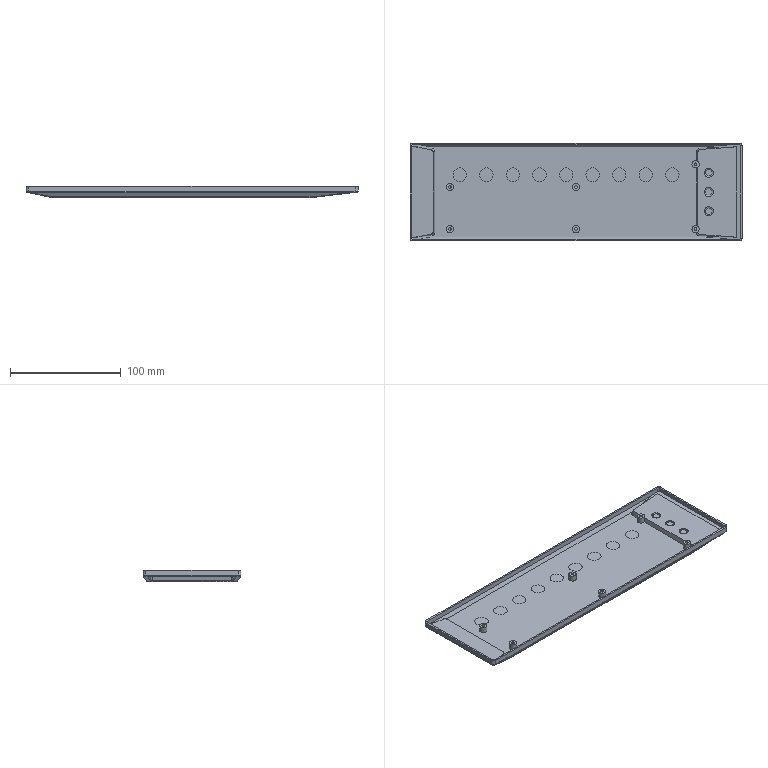NC program | NX | posted with a generic post | part box 300 x 88.5 x 10 mm
Lines 23 to 1103 of 32249:
(ADAPTIVE_MILLING , TOOL : D8)
N44 T08 M6
N46 G54
N48 G17 G0 G90 X-161.13 Y0.006 S9500 M3
N50 G43 Z30. H8
N52 Z-7.
N54 G94 G1 Z-10. F1000.
N56 X-159.864 Y-0.423 F3000.
N58 G3 X-159.003 Y0.006 R0.814
N60 X-158.379 Y2.947 R8.132
N62 X-158.203 Y14.163 R185.26
N64 G1 X-158.202 Y22.083
N66 X-158.201 Y46.803
N68 X-158.2 Y46.923
N70 X-158.195 Y47.043
N72 X-158.191 Y47.103
N74 X-158.179 Y47.223
N76 G2 X-155.684 Y50.713 R4.933
N78 X-150.774 Y52.157 R11.806
N80 X-141.902 Y52.427 R96.276
N82 G1 X-139.742 Y52.431
N84 X-135.542 Y52.434
N86 X-53.462 Y52.435
N88 X-52.982 Y52.437
N90 X-52.142 Y52.438
N92 X-51.722
N94 X-51.242 Y52.44
N96 X-50.282
N98 X-49.742 Y52.441
N100 X-48.722 Y52.44
N102 X-48.182 Y52.442
N104 X-47.222 Y52.441
N106 X-46.742 Y52.442
N108 X-45.902 Y52.441
N110 X-45.542
N112 X-45.002 Y52.442
N114 X-43.982 Y52.441
N116 X-43.442 Y52.443
N118 X-42.482 Y52.441
N120 X-41.822 Y52.443
N122 X-41.222
N124 X-40.382 Y52.444
N126 X-39.842 Y52.443
N128 X-38.942 Y52.444
N130 X-38.462
N132 X-37.382 Y52.445
N134 X-36.902 Y52.444
N136 X-35.882 Y52.445
N138 X-35.402 Y52.444
N140 X-34.442 Y52.445
N142 X-33.902 Y52.444
N144 X-32.942 Y52.445
N146 X-32.282 Y52.444
N148 X-31.382 Y52.446
N150 X-30.902 Y52.445
N152 X-29.522 Y52.446
N154 X-29.162
N156 X-28.742 Y52.445
N158 X-27.722 Y52.446
N160 X-27.122 Y52.444
N162 X-26.402 Y52.445
N164 X-25.802 Y52.444
N166 X-24.902 Y52.445
N168 X-24.302 Y52.444
N170 X-23.642 Y52.445
N172 X-23.042 Y52.443
N174 X-22.262 Y52.445
N176 X-21.782 Y52.444
N178 X-20.822 Y52.445
N180 X-20.342 Y52.444
N182 X-19.442 Y52.445
N184 X-18.962 Y52.444
N186 X-18.122 Y52.445
N188 X-17.582 Y52.444
N190 X-16.682 Y52.445
N192 X-16.202 Y52.444
N194 X-15.062 Y52.445
N196 X-14.582
N198 X-13.682 Y52.446
N200 X-13.322
N202 X-12.782 Y52.444
N204 X-12.002 Y52.445
N206 X-11.522 Y52.444
N208 X-10.502 Y52.445
N210 X-9.962 Y52.444
N212 X-9.182 Y52.445
N214 X-8.642 Y52.444
N216 X-7.742 Y52.445
N218 X-7.082 Y52.443
N220 X-6.242 Y52.445
N222 X-5.762 Y52.444
N224 X-4.802 Y52.445
N226 X-4.262 Y52.444
N228 X-3.422 Y52.445
N230 X-2.882 Y52.444
N232 X-1.922 Y52.445
N234 X-1.262 Y52.443
N236 X-0.422 Y52.445
N238 X0.118 Y52.444
N240 X1.078 Y52.445
N242 X1.618 Y52.444
N244 X2.518 Y52.445
N246 X2.998 Y52.444
N248 X4.138 Y52.446
N250 X4.618 Y52.445
N252 X5.518 Y52.446
N254 X5.878
N256 X6.358 Y52.444
N258 X7.258 Y52.445
N260 X7.738
N262 X8.818 Y52.446
N264 X9.298 Y52.444
N266 X10.258 Y52.445
N268 X10.798 Y52.444
N270 X11.578 Y52.445
N272 X12.118 Y52.444
N274 X13.078 Y52.445
N276 X13.738 Y52.443
N278 X14.338 Y52.444
N280 X15.178 Y52.443
N282 X15.778 Y52.444
N284 X16.618 Y52.442
N286 X17.098 Y52.443
N288 X18.238 Y52.442
N290 X18.718 Y52.443
N292 X19.798 Y52.441
N294 X20.338 Y52.443
N296 X21.178 Y52.442
N298 X21.718 Y52.443
N300 X22.738 Y52.442
N302 X23.278 Y52.443
N304 X24.238 Y52.442
N306 X24.718
N308 X25.918 Y52.441
N310 X26.578 Y52.443
N312 X27.418 Y52.441
N314 X27.898 Y52.442
N316 X28.798 Y52.441
N318 X29.158
N320 X29.578 Y52.442
N322 X30.718 Y52.441
N324 X31.198 Y52.442
N326 X32.218 Y52.441
N328 X32.758 Y52.443
N330 X33.718 Y52.441
N332 X34.378 Y52.443
N334 X34.978
N336 X35.818 Y52.444
N338 X36.418 Y52.443
N340 X37.198 Y52.444
N342 X37.678 Y52.443
N344 X38.698 Y52.445
N346 X39.298 Y52.443
N348 X40.078 Y52.445
N350 X40.558 Y52.444
N352 X41.698 Y52.445
N354 X42.358 Y52.444
N356 X43.198 Y52.445
N358 X43.678 Y52.444
N360 X44.818 Y52.445
N362 X45.298 Y52.444
N364 X46.198 Y52.445
N366 X46.738 Y52.444
N368 X47.698 Y52.445
N370 X48.358 Y52.444
N372 X49.198 Y52.445
N374 X49.678 Y52.444
N376 X50.818 Y52.445
N378 X51.358 Y52.444
N380 X52.138 Y52.445
N382 X52.678 Y52.444
N384 X53.638 Y52.445
N386 X54.238 Y52.444
N388 X54.958 Y52.445
N390 X55.618 Y52.443
N392 X56.278 Y52.444
N394 X57.118 Y52.443
N396 X57.718 Y52.444
N398 X58.438 Y52.443
N400 X59.098 Y52.444
N402 X59.698 Y52.443
N404 X60.418 Y52.444
N406 X61.078 Y52.443
N408 X61.678 Y52.444
N410 X62.398 Y52.443
N412 X63.058 Y52.444
N414 X63.718 Y52.443
N416 X64.558 Y52.445
N418 X65.158 Y52.443
N420 X65.938 Y52.444
N422 X66.418 Y52.443
N424 X67.378 Y52.445
N426 X67.978 Y52.443
N428 X68.758 Y52.445
N430 X69.238 Y52.444
N432 X70.258 Y52.445
N434 X70.858 Y52.444
N436 X71.638 Y52.445
N438 X72.118 Y52.444
N440 X73.138 Y52.445
N442 X73.738 Y52.444
N444 X74.578 Y52.445
N446 X75.058 Y52.444
N448 X76.258 Y52.446
N450 X76.858 Y52.444
N452 X77.578 Y52.445
N454 X78.178 Y52.444
N456 X79.138 Y52.445
N458 X79.678 Y52.444
N460 X80.698 Y52.445
N462 X81.238 Y52.444
N464 X82.138 Y52.445
N466 X82.618 Y52.444
N468 X83.698 Y52.445
N470 X84.178 Y52.444
N472 X85.138 Y52.445
N474 X85.618 Y52.444
N476 X86.578 Y52.445
N478 X87.058 Y52.444
N480 X88.018 Y52.445
N482 X88.498 Y52.444
N484 X89.458 Y52.445
N486 X89.938 Y52.444
N488 X90.898 Y52.445
N490 X91.438 Y52.444
N492 X92.218 Y52.445
N494 X92.758 Y52.444
N496 X93.658 Y52.445
N498 X94.318 Y52.443
N500 X95.158 Y52.445
N502 X95.698 Y52.444
N504 X96.478
N506 X97.018 Y52.443
N508 X97.918 Y52.445
N510 X98.518 Y52.443
N512 X99.238 Y52.444
N514 X99.838 Y52.443
N516 X100.738 Y52.445
N518 X101.338 Y52.443
N520 X102.058 Y52.444
N522 X102.718 Y52.443
N524 X103.378 Y52.444
N526 X104.158 Y52.443
N528 X104.758 Y52.444
N530 X105.418 Y52.443
N532 X106.018 Y52.444
N534 X106.798 Y52.443
N536 X107.278
N538 X108.238 Y52.442
N540 X108.778 Y52.443
N542 X109.738 Y52.442
N544 X110.338 Y52.443
N546 X110.998 Y52.442
N548 X111.598 Y52.443
N550 X112.378 Y52.442
N552 X112.798 Y52.443
N554 X113.818 Y52.442
N556 X114.358 Y52.443
N558 X115.378 Y52.442
N560 X115.918 Y52.443
N562 X116.878 Y52.442
N564 X117.358
N566 X118.558 Y52.441
N568 X119.218 Y52.443
N570 X120.058 Y52.441
N572 X120.538 Y52.442
N574 X121.438 Y52.441
N576 X121.798
N578 X122.218 Y52.442
N580 X123.358 Y52.441
N582 X123.838 Y52.442
N584 X124.858 Y52.441
N586 X125.398 Y52.443
N588 X126.358 Y52.441
N590 X127.018 Y52.443
N592 X127.618
N594 X128.458 Y52.444
N596 X129.058 Y52.443
N598 X129.838 Y52.444
N600 X130.318
N602 X131.338 Y52.445
N604 X131.938 Y52.443
N606 X132.718 Y52.445
N608 X133.198 Y52.444
N610 X134.278 Y52.445
N612 X134.758 Y52.444
N614 X135.838 Y52.446
N616 X136.318 Y52.444
N618 X137.338 Y52.446
N620 X137.818 Y52.444
N622 X138.778 Y52.445
N624 X139.318 Y52.444
N626 X140.338 Y52.445
N628 X140.938 Y52.444
N630 X141.718 Y52.445
N632 X142.198 Y52.444
N634 X143.278 Y52.445
N636 X143.758
N638 X144.778
N640 X145.318 Y52.444
N642 X146.278 Y52.445
N644 X146.878 Y52.444
N646 X147.538 Y52.445
N648 X148.138 Y52.444
N650 X148.918 Y52.445
N652 X149.338 Y52.444
N654 X150.358 Y52.445
N656 X150.898 Y52.444
N658 X151.678
N660 X152.158
N662 X152.578
N664 X152.698 Y52.443
N666 X152.758 Y52.44
N668 X152.877 Y52.432
N670 X152.937 Y52.426
N672 G2 X156.508 Y49.856 R4.952
N674 X157.935 Y44.755 R12.252
N676 X158.178 Y35.341 R114.229
N678 G1 X158.182 Y32.641
N680 X158.183 Y25.681
N682 X158.184 Y-18.779
N684 X158.186 Y-19.259
N686 X158.187 Y-20.099
N688 Y-20.519
N690 X158.189 Y-20.999
N692 Y-21.959
N694 X158.191 Y-22.499
N696 X158.19 Y-23.519
N698 X158.191 Y-24.059
N700 X158.19 Y-25.139
N702 X158.191 Y-25.559
N704 X158.19 Y-26.399
N706 Y-26.759
N708 X158.192 Y-27.359
N710 X158.191 Y-28.019
N712 X158.193 Y-28.859
N714 X158.192 Y-29.399
N716 X158.193 Y-30.299
N718 X158.192 Y-30.959
N720 X158.194 Y-31.739
N722 X158.192 Y-32.279
N724 X158.194 Y-33.179
N726 X158.192 Y-33.779
N728 X158.193 Y-34.439
N730 X158.192 Y-35.279
N732 X158.193 Y-35.879
N734 G2 X158.164 Y-47.277 R562.013
N736 X155.574 Y-50.772 R5.009
N738 X150.529 Y-52.182 R12.239
N740 X141.416 Y-52.428 R108.49
N742 G1 X138.896 Y-52.432
N744 X133.316 Y-52.434
N746 X28.196 Y-52.435
N748 X27.776 Y-52.436
N750 X25.976 Y-52.44
N752 X24.236 Y-52.439
N754 X23.696
N756 X23.156 Y-52.441
N758 X22.196 Y-52.44
N760 X21.716 Y-52.442
N762 X20.876 Y-52.441
N764 X20.396 Y-52.442
N766 X19.436 Y-52.441
N768 X18.956 Y-52.442
N770 X17.816 Y-52.441
N772 X17.336 Y-52.442
N774 X16.496
N776 X16.016 Y-52.443
N778 X14.996 Y-52.441
N780 X14.516 Y-52.442
N782 X13.316 Y-52.441
N784 X12.836 Y-52.442
N786 X11.816 Y-52.441
N788 X11.216 Y-52.443
N790 X10.256 Y-52.441
N792 X9.716 Y-52.443
N794 X8.936 Y-52.442
N796 X8.396 Y-52.443
N798 X7.496 Y-52.442
N800 X6.896 Y-52.443
N802 X6.116 Y-52.442
N804 X5.636 Y-52.443
N806 X4.616 Y-52.442
N808 X4.076 Y-52.443
N810 X3.356 Y-52.442
N812 X2.816 Y-52.443
N814 X2.036 Y-52.442
N816 X1.436 Y-52.444
N818 X0.536 Y-52.442
N820 X0.056 Y-52.443
N822 X-0.964 Y-52.442
N824 X-1.384
N826 X-1.804 Y-52.443
N828 X-2.584 Y-52.442
N830 X-3.064 Y-52.443
N832 X-4.084 Y-52.442
N834 X-4.684 Y-52.443
N836 X-5.584 Y-52.442
N838 X-6.064 Y-52.443
N840 X-7.204 Y-52.442
N842 X-7.684 Y-52.443
N844 X-8.584 Y-52.442
N846 X-9.184 Y-52.443
N848 X-10.024 Y-52.442
N850 X-10.504 Y-52.443
N852 X-11.404 Y-52.442
N854 X-11.764 Y-52.441
N856 X-12.304 Y-52.443
N858 X-13.144 Y-52.442
N860 X-13.744 Y-52.443
N862 X-14.644 Y-52.442
N864 X-15.304 Y-52.444
N866 X-16.144 Y-52.442
N868 X-16.684 Y-52.443
N870 X-17.704 Y-52.442
N872 X-18.304 Y-52.443
N874 X-19.204 Y-52.442
N876 X-19.864 Y-52.444
N878 X-20.464 Y-52.443
N880 X-21.304 Y-52.444
N882 X-21.964 Y-52.443
N884 X-22.624 Y-52.444
N886 X-23.284 Y-52.443
N888 X-23.944 Y-52.444
N890 X-24.544 Y-52.443
N892 X-25.444 Y-52.445
N894 X-25.924 Y-52.444
N896 X-27.124 Y-52.445
N898 X-27.784 Y-52.444
N900 X-28.624 Y-52.445
N902 X-29.164 Y-52.444
N904 X-30.184 Y-52.445
N906 X-30.784 Y-52.444
N908 X-31.744 Y-52.445
N910 X-32.344 Y-52.444
N912 X-33.184 Y-52.445
N914 X-33.664 Y-52.444
N916 X-34.564 Y-52.445
N918 X-34.924
N920 X-35.524 Y-52.444
N922 X-36.124
N924 X-37.024 Y-52.443
N926 X-37.564 Y-52.444
N928 X-38.404 Y-52.443
N930 X-39.004 Y-52.444
N932 X-39.904 Y-52.442
N934 X-40.564 Y-52.444
N936 X-41.404 Y-52.442
N938 X-42.004 Y-52.443
N940 X-42.844 Y-52.442
N942 X-43.444 Y-52.444
N944 X-44.344 Y-52.442
N946 X-44.824 Y-52.443
N948 X-45.844 Y-52.442
N950 X-46.264
N952 X-46.684 Y-52.443
N954 X-47.464 Y-52.442
N956 X-47.944 Y-52.443
N958 X-48.904 Y-52.442
N960 X-49.504 Y-52.443
N962 X-50.404 Y-52.442
N964 X-50.884 Y-52.443
N966 X-51.904 Y-52.441
N968 X-52.324 Y-52.442
N970 X-52.744 Y-52.443
N972 X-53.524 Y-52.442
N974 X-54.004 Y-52.443
N976 X-55.024 Y-52.442
N978 X-55.564 Y-52.443
N980 X-56.344 Y-52.442
N982 X-56.944 Y-52.444
N984 X-57.784 Y-52.442
N986 X-58.264 Y-52.443
N988 X-59.164 Y-52.442
N990 X-59.704 Y-52.443
N992 X-60.424
N994 X-60.964 Y-52.444
N996 X-61.744 Y-52.442
N998 X-62.284 Y-52.444
N1000 X-63.244 Y-52.442
N1002 X-63.724 Y-52.443
N1004 X-64.924 Y-52.441
N1006 X-65.584 Y-52.443
N1008 X-66.184
N1010 X-67.084 Y-52.444
N1012 X-67.684 Y-52.443
N1014 X-68.584 Y-52.445
N1016 X-69.304 Y-52.443
N1018 X-70.024 Y-52.444
N1020 X-70.564
N1022 X-71.524 Y-52.445
N1024 X-72.124 Y-52.443
N1026 X-72.904 Y-52.445
N1028 X-73.384 Y-52.444
N1030 X-74.404 Y-52.445
N1032 X-75.004 Y-52.444
N1034 X-75.784 Y-52.445
N1036 X-76.264 Y-52.444
N1038 X-77.284 Y-52.445
N1040 X-77.884 Y-52.444
N1042 X-78.724 Y-52.445
N1044 X-79.204 Y-52.444
N1046 X-80.404 Y-52.446
N1048 X-81.004 Y-52.444
N1050 X-81.784 Y-52.445
N1052 X-82.264 Y-52.444
N1054 X-83.284 Y-52.445
N1056 X-83.824 Y-52.444
N1058 X-84.544 Y-52.445
N1060 X-85.084 Y-52.444
N1062 X-85.864 Y-52.445
N1064 X-86.404 Y-52.443
N1066 X-87.304 Y-52.445
N1068 X-87.784 Y-52.444
N1070 X-88.984 Y-52.446
N1072 X-89.584 Y-52.444
N1074 X-90.364 Y-52.445
N1076 X-90.844 Y-52.444
N1078 X-91.924 Y-52.445
N1080 X-92.404 Y-52.444
N1082 X-93.244 Y-52.445
N1084 X-93.724 Y-52.444
N1086 X-94.684 Y-52.445
N1088 X-95.344 Y-52.444
N1090 X-96.184 Y-52.445
N1092 X-96.724 Y-52.444
N1094 X-97.744 Y-52.445
N1096 X-98.344 Y-52.444
N1098 X-99.304 Y-52.445
N1100 X-99.904 Y-52.444
N1102 X-100.744 Y-52.445
N1104 X-101.224 Y-52.444
N1106 X-102.364 Y-52.445
N1108 X-102.844 Y-52.444
N1110 X-103.684 Y-52.445
N1112 X-104.164 Y-52.444
N1114 X-105.184 Y-52.445
N1116 X-105.844 Y-52.444
N1118 X-106.444
N1120 X-107.284 Y-52.443
N1122 X-107.884 Y-52.444
N1124 X-108.724 Y-52.443
N1126 X-109.204
N1128 X-110.344 Y-52.442
N1130 X-110.824 Y-52.443
N1132 X-111.664 Y-52.442
N1134 X-112.144 Y-52.443
N1136 X-113.164 Y-52.442
N1138 X-113.824 Y-52.443
N1140 X-114.424
N1142 X-115.264 Y-52.444
N1144 X-115.864 Y-52.443
N1146 X-116.644 Y-52.444
N1148 X-117.124
N1150 X-118.144 Y-52.445
N1152 X-118.744 Y-52.443
N1154 X-119.524 Y-52.445
N1156 X-120.004 Y-52.444
N1158 X-121.024 Y-52.445
N1160 X-121.684 Y-52.443
N1162 X-122.344 Y-52.445
N1164 X-122.944 Y-52.443
N1166 X-123.904 Y-52.445
N1168 X-124.504 Y-52.444
N1170 X-125.284 Y-52.445
N1172 X-125.764 Y-52.444
N1174 X-126.784 Y-52.445
N1176 X-127.324 Y-52.444
N1178 X-128.104 Y-52.445
N1180 X-128.704 Y-52.443
N1182 X-129.484 Y-52.445
N1184 X-129.964 Y-52.444
N1186 X-130.804
N1188 X-131.284
N1190 X-132.304 Y-52.445
N1192 X-132.784 Y-52.444
N1194 X-133.984 Y-52.445
N1196 X-134.464 Y-52.444
N1198 X-135.424 Y-52.445
N1200 X-136.024 Y-52.444
N1202 X-136.804 Y-52.445
N1204 X-137.284 Y-52.444
N1206 X-138.304 Y-52.445
N1208 X-138.904 Y-52.444
N1210 G2 X-153.003 Y-52.418 R834.45
N1212 X-156.539 Y-49.793 R5.021
N1214 X-157.942 Y-44.684 R12.482
N1216 X-158.179 Y-35.09 R120.129
N1218 G1 X-158.182 Y-32.09
N1220 X-158.183 Y-23.09
N1222 Y-3.05
N1224 X-158.181 Y-2.87
N1226 X-158.173 Y-2.63
N1228 X-158.161 Y-2.39
N1230 G3 X-157.554 Y4.24 R142.602
N1232 X-157.412 Y17.858 R382.618
N1234 G1 X-157.411 Y30.758
N1236 Y44.378
N1238 X-157.409 Y44.498
N1240 X-157.405 Y44.618
N1242 X-157.398 Y44.738
N1244 X-157.395 Y44.798
N1246 G2 X-154.043 Y49.756 R6.28
N1248 X-148.421 Y51.328 R14.21
N1250 X-138.829 Y51.617 R108.831
N1252 G1 X-136.669 Y51.622
N1254 X-132.889 Y51.624
N1256 X-112.789 Y51.625
N1258 X-55.849
N1260 X-55.309 Y51.629
N1262 X-54.349 Y51.631
N1264 X-53.989
N1266 X-53.449 Y51.634
N1268 X-52.549 Y51.635
N1270 X-51.889 Y51.637
N1272 X-50.989
N1274 X-50.449 Y51.639
N1276 X-49.489 Y51.638
N1278 X-48.949 Y51.64
N1280 X-47.929 Y51.639
N1282 X-47.329 Y51.64
N1284 X-46.369 Y51.639
N1286 X-45.709 Y51.641
N1288 X-44.809 Y51.64
N1290 X-44.089 Y51.642
N1292 X-43.489 Y51.641
N1294 X-42.709 Y51.643
N1296 X-41.929 Y51.641
N1298 X-41.209 Y51.644
N1300 X-40.369 Y51.642
N1302 X-39.769 Y51.644
N1304 X-38.869 Y51.643
N1306 X-38.149 Y51.645
N1308 X-37.549 Y51.644
N1310 X-36.769 Y51.645
N1312 X-36.109 Y51.644
N1314 X-35.209 Y51.646
N1316 X-34.609 Y51.644
N1318 X-33.709 Y51.646
N1320 X-33.109 Y51.644
N1322 X-31.969 Y51.647
N1324 X-31.129 Y51.644
N1326 X-30.169 Y51.647
N1328 X-29.449 Y51.645
N1330 X-28.609 Y51.646
N1332 X-28.009 Y51.645
N1334 X-27.109 Y51.646
N1336 X-26.509 Y51.645
N1338 X-25.669
N1340 X-25.129 Y51.644
N1342 X-24.349 Y51.645
N1344 X-23.749 Y51.644
N1346 X-23.029 Y51.645
N1348 X-22.189 Y51.643
N1350 X-21.709 Y51.644
N1352 X-20.749 Y51.643
N1354 X-20.269 Y51.644
N1356 X-19.369 Y51.643
N1358 X-18.769 Y51.644
N1360 X-17.869 Y51.643
N1362 X-17.329 Y51.644
N1364 X-16.369 Y51.643
N1366 X-15.709 Y51.645
N1368 X-14.989 Y51.644
N1370 X-14.149 Y51.646
N1372 X-13.549 Y51.644
N1374 X-12.769 Y51.646
N1376 X-12.109 Y51.644
N1378 X-11.449 Y51.645
N1380 X-10.729 Y51.644
N1382 X-10.069 Y51.645
N1384 X-9.289 Y51.644
N1386 X-8.569 Y51.645
N1388 X-7.969 Y51.644
N1390 X-7.129 Y51.645
N1392 X-6.589 Y51.644
N1394 X-5.689 Y51.645
N1396 X-5.089 Y51.644
N1398 X-4.189 Y51.646
N1400 X-3.469 Y51.644
N1402 X-2.749 Y51.645
N1404 X-2.089 Y51.644
N1406 X-1.189 Y51.646
N1408 X-0.589 Y51.644
N1410 X0.191 Y51.645
N1412 X0.911 Y51.644
N1414 X1.751 Y51.646
N1416 X2.351 Y51.645
N1418 X3.431 Y51.647
N1420 X4.151 Y51.645
N1422 X4.811 Y51.646
N1424 X5.591 Y51.645
N1426 X6.431 Y51.647
N1428 X6.971 Y51.646
N1430 X8.231 Y51.647
N1432 X8.591
N1434 X9.071 Y51.646
N1436 X10.211 Y51.647
N1438 X10.631 Y51.646
N1440 X11.951 Y51.648
N1442 X12.371 Y51.646
N1444 X13.451 Y51.647
N1446 X13.811
N1448 X14.291 Y51.645
N1450 X15.251 Y51.646
N1452 X15.911 Y51.644
N1454 X16.871 Y51.645
N1456 X17.411 Y51.643
N1458 X18.371 Y51.644
N1460 X18.911 Y51.643
N1462 X19.811
N1464 X20.471 Y51.642
N1466 X21.071 Y51.643
N1468 X21.911 Y51.642
N1470 X22.511 Y51.643
N1472 X23.291 Y51.642
N1474 X24.191 Y51.644
N1476 X25.091 Y51.641
N1478 X25.871 Y51.643
N1480 X26.711 Y51.641
N1482 X27.431 Y51.643
N1484 X28.331 Y51.64
N1486 X28.871 Y51.641
N1488 X30.191 Y51.64
N1490 X30.551
N1492 X31.031 Y51.641
N1494 X31.871 Y51.64
N1496 X32.291 Y51.641
N1498 X33.251
N1500 X33.731 Y51.642
N1502 X34.511
N1504 X34.991 Y51.643
N1506 X35.891 Y51.642
N1508 X36.431 Y51.643
N1510 X37.391 Y51.642
N1512 X37.931 Y51.644
N1514 X38.891 Y51.642
N1516 X39.431 Y51.644
N1518 X40.391 Y51.643
N1520 X40.811
N1522 X41.171 Y51.644
N1524 X42.071 Y51.643
N1526 X42.551 Y51.644
N1528 X43.571 Y51.643
N1530 X44.051 Y51.644
N1532 X44.951 Y51.643
N1534 X45.551 Y51.645
N1536 X46.331 Y51.643
N1538 X46.991 Y51.645
N1540 X47.771 Y51.644
N1542 X48.311 Y51.645
N1544 X49.391 Y51.643
N1546 X49.931 Y51.644
N1548 X50.891 Y51.643
N1550 X51.491 Y51.645
N1552 X52.331 Y51.643
N1554 X52.871 Y51.644
N1556 X53.711 Y51.643
N1558 X54.251 Y51.644
N1560 X55.091 Y51.643
N1562 X55.631 Y51.644
N1564 X56.411 Y51.643
N1566 X56.951 Y51.644
N1568 X57.671 Y51.643
N1570 X58.331 Y51.644
N1572 X58.991 Y51.643
N1574 X59.771 Y51.644
N1576 X60.311 Y51.643
N1578 X61.151 Y51.644
N1580 X61.691 Y51.643
N1582 X62.531 Y51.644
N1584 X63.071 Y51.643
N1586 X63.911 Y51.644
N1588 X64.391
N1590 X65.231 Y51.645
N1592 X65.831 Y51.643
N1594 X66.611 Y51.644
N1596 X67.151
N1598 X67.931 Y51.645
N1600 X68.531 Y51.644
N1602 X69.311 Y51.645
N1604 X69.971 Y51.644
N1606 X70.811 Y51.645
N1608 X71.471 Y51.644
N1610 X72.191 Y51.645
N1612 X72.971 Y51.644
N1614 X73.811 Y51.646
N1616 X74.651 Y51.644
N1618 X75.371 Y51.645
N1620 X76.031 Y51.644
N1622 X76.871 Y51.646
N1624 X77.591 Y51.644
N1626 X78.371 Y51.646
N1628 X79.031 Y51.644
N1630 X79.751 Y51.645
N1632 X80.471 Y51.644
N1634 X81.311 Y51.646
N1636 X81.851 Y51.645
N1638 X83.111 Y51.647
N1640 X83.531
N1642 X84.011 Y51.646
N1644 X84.851 Y51.647
N1646 X85.331 Y51.645
N1648 X86.111 Y51.646
N1650 X86.651 Y51.645
N1652 X87.431 Y51.646
N1654 X87.911 Y51.645
N1656 X88.811 Y51.646
N1658 X89.291 Y51.645
N1660 X90.191 Y51.646
N1662 X90.791 Y51.644
N1664 X91.631 Y51.646
N1666 X92.231 Y51.644
N1668 X93.071 Y51.645
N1670 X93.611 Y51.644
N1672 X94.511 Y51.645
N1674 X95.051 Y51.644
N1676 X95.831 Y51.645
N1678 X96.491 Y51.643
N1680 X97.151 Y51.644
N1682 X97.991 Y51.643
N1684 X98.531 Y51.644
N1686 X99.551 Y51.643
N1688 X100.091 Y51.644
N1690 X100.871 Y51.643
N1692 X101.291 Y51.644
N1694 X102.311 Y51.642
N1696 X102.791 Y51.643
N1698 X103.571
N1700 X103.991
N1702 X104.951 Y51.642
N1704 X105.491 Y51.643
N1706 X106.271 Y51.642
N1708 X106.751 Y51.643
N1710 X107.591 Y51.642
N1712 X108.191 Y51.643
N1714 X109.03 Y51.642
N1716 X109.57 Y51.643
N1718 X110.53 Y51.642
N1720 X111.01
N1722 X112.15 Y51.641
N1724 X112.63 Y51.642
N1726 X113.41 Y51.641
N1728 X113.95 Y51.643
N1730 X114.79 Y51.641
N1732 X115.27 Y51.642
N1734 X116.23 Y51.641
N1736 X117.01 Y51.643
N1738 X117.61 Y51.642
N1740 X118.51 Y51.643
N1742 X119.23 Y51.641
N1744 X119.83 Y51.642
N1746 X120.79 Y51.641
N1748 X121.51 Y51.642
N1750 X122.23 Y51.641
N1752 X123.07 Y51.643
N1754 X123.97 Y51.641
N1756 X124.75 Y51.643
N1758 X125.29 Y51.642
N1760 X126.61 Y51.644
N1762 X127.09 Y51.643
N1764 X128.05 Y51.645
N1766 X128.53 Y51.644
N1768 X129.49 Y51.645
N1770 X129.97 Y51.644
N1772 X130.87 Y51.645
N1774 X131.35 Y51.644
N1776 X132.25 Y51.645
N1778 X132.91 Y51.644
N1780 X133.63 Y51.646
N1782 X134.29 Y51.644
N1784 X135.01 Y51.645
N1786 X135.73 Y51.644
N1788 X136.45 Y51.646
N1790 X137.05 Y51.645
N1792 X137.95 Y51.646
N1794 X138.67 Y51.644
N1796 X139.39 Y51.646
N1798 X140.05 Y51.644
N1800 G2 X150.789 Y51.607 R349.934
N1802 X155.51 Y48.28 R6.322
N1804 X157.064 Y42.776 R13.989
N1806 X157.363 Y33.905 R96.634
N1808 G1 X157.369 Y32.105
N1810 X157.372 Y29.345
N1812 X157.374 Y23.225
N1814 X157.375 Y-16.375
N1816 X157.377 Y-16.855
N1818 X157.38 Y-18.055
N1820 X157.381 Y-18.715
N1822 X157.383 Y-19.195
N1824 X157.384 Y-19.975
N1826 X157.386 Y-20.395
N1828 Y-21.235
N1830 X157.388 Y-21.775
N1832 X157.387 Y-22.735
N1834 X157.389 Y-23.275
N1836 X157.388 Y-23.935
N1838 Y-24.415
N1840 X157.389 Y-24.955
N1842 Y-25.855
N1844 X157.391 Y-26.515
N1846 X157.39 Y-27.415
N1848 X157.391 Y-27.955
N1850 Y-28.915
N1852 X157.392 Y-29.515
N1854 X157.391 Y-30.355
N1856 X157.392 Y-30.895
N1858 X157.391 Y-31.735
N1860 Y-32.095
N1862 X157.392 Y-32.515
N1864 X157.391 Y-33.355
N1866 X157.392 Y-33.835
N1868 G2 X157.36 Y-44.994 R456.705
N1870 X153.96 Y-49.795 R6.334
N1872 X148.269 Y-51.341 R14.472
N1874 X137.596 Y-51.62 R126.976
N1876 G1 X134.656 Y-51.623
N1878 X127.396 Y-51.625
N1880 X30.616
N1882 X30.136 Y-51.628
N1884 X28.396 Y-51.632
N1886 X26.716 Y-51.633
N1888 X26.116
N1890 X25.576 Y-51.635
N1892 X24.616 Y-51.636
N1894 X24.136 Y-51.637
N1896 X23.776 Y-51.638
N1898 X23.056
N1900 X22.516 Y-51.64
N1902 X21.616 Y-51.639
N1904 X21.016 Y-51.641
N1906 X20.116 Y-51.64
N1908 X19.576 Y-51.641
N1910 X18.616 Y-51.64
N1912 X18.016 Y-51.642
N1914 X17.237 Y-51.641
N1916 X16.637 Y-51.642
N1918 X15.677 Y-51.64
N1920 X15.017 Y-51.642
N1922 X14.117 Y-51.64
N1924 X13.397 Y-51.642
N1926 X12.497 Y-51.64
N1928 X11.957 Y-51.642
N1930 X11.057 Y-51.641
N1932 X10.577 Y-51.642
N1934 X9.617 Y-51.641
N1936 X8.957 Y-51.643
N1938 X8.297 Y-51.642
N1940 X7.577 Y-51.643
N1942 X6.857 Y-51.641
N1944 X6.257 Y-51.642
N1946 X5.357
N1948 X4.817 Y-51.643
N1950 X3.977 Y-51.642
N1952 X3.497
N1954 X2.417 Y-51.641
N1956 X1.937 Y-51.642
N1958 X0.977 Y-51.641
N1960 X0.317 Y-51.643
N1962 X-0.403 Y-51.641
N1964 X-1.063 Y-51.643
N1966 X-1.903 Y-51.641
N1968 X-2.443 Y-51.642
N1970 X-3.583 Y-51.641
N1972 X-4.123 Y-51.642
N1974 X-5.023 Y-51.641
N1976 X-5.563 Y-51.642
N1978 X-6.463 Y-51.641
N1980 X-7.003 Y-51.642
N1982 X-7.903 Y-51.641
N1984 X-8.383 Y-51.642
N1986 X-9.403 Y-51.641
N1988 X-10.243 Y-51.643
N1990 X-10.843 Y-51.641
N1992 X-11.623 Y-51.643
N1994 X-12.283 Y-51.641
N1996 X-13.003 Y-51.643
N1998 X-13.783 Y-51.641
N2000 X-14.443 Y-51.643
N2002 X-15.343 Y-51.641
N2004 X-15.883 Y-51.642
N2006 X-16.903 Y-51.641
N2008 X-17.623 Y-51.642
N2010 X-18.643 Y-51.641
N2012 X-19.183 Y-51.643
N2014 X-20.083 Y-51.642
N2016 X-20.563 Y-51.643
N2018 X-21.463 Y-51.642
N2020 X-22.003 Y-51.643
N2022 X-22.723
N2024 X-23.383 Y-51.644
N2026 X-24.043 Y-51.643
N2028 X-24.763 Y-51.645
N2030 X-25.603 Y-51.643
N2032 X-26.263 Y-51.645
N2034 X-26.983 Y-51.644
N2036 X-27.823 Y-51.646
N2038 X-28.423 Y-51.644
N2040 X-29.263 Y-51.645
N2042 X-30.103 Y-51.643
N2044 X-30.823 Y-51.645
N2046 X-31.423 Y-51.644
N2048 X-32.503 Y-51.646
N2050 X-33.283 Y-51.644
N2052 X-33.823 Y-51.645
N2054 X-34.783 Y-51.643
N2056 X-35.503 Y-51.645
N2058 X-36.223 Y-51.643
N2060 X-36.823 Y-51.644
N2062 X-37.663 Y-51.643
N2064 X-38.263 Y-51.644
N2066 X-39.163 Y-51.642
N2068 X-39.883 Y-51.644
N2070 X-40.603 Y-51.642
N2072 X-41.203 Y-51.643
N2074 X-42.163 Y-51.642
N2076 X-42.883 Y-51.643
N2078 X-43.723 Y-51.641
N2080 X-44.503 Y-51.643
N2082 X-45.103 Y-51.642
N2084 X-46.003 Y-51.643
N2086 X-46.603 Y-51.642
N2088 X-47.443 Y-51.643
N2090 X-48.043 Y-51.642
N2092 X-48.883 Y-51.643
N2094 X-49.423 Y-51.642
N2096 X-50.383 Y-51.644
N2098 X-51.103 Y-51.642
N2100 X-51.703 Y-51.643
N2102 X-52.543 Y-51.642
N2104 X-53.203 Y-51.643
N2106 X-54.103 Y-51.641
N2108 X-54.643 Y-51.642
N2110 X-55.783 Y-51.641
N2112 X-56.263 Y-51.642
N2114 X-57.103 Y-51.641
N2116 X-57.703 Y-51.643
N2118 X-58.423 Y-51.642
N2120 X-58.963 Y-51.643
N2122 X-59.743 Y-51.642
N2124 X-60.223 Y-51.643
N2126 X-61.123 Y-51.642
N2128 X-61.603 Y-51.643
N2130 X-62.623 Y-51.641
N2132 X-63.283 Y-51.643
N2134 X-64.183 Y-51.641
N2136 X-64.783 Y-51.643
N2138 X-65.563 Y-51.642
N2140 X-66.223 Y-51.644
N2142 X-67.063 Y-51.642
N2144 X-67.783 Y-51.644
N2146 X-68.503 Y-51.643
N2148 X-69.283 Y-51.645
N2150 X-70.003 Y-51.643
N2152 X-70.723 Y-51.645
N2154 X-71.383 Y-51.643
N2156 X-72.043 Y-51.645
N2158 X-72.943 Y-51.643
N2160 X-73.483 Y-51.644
N2162 X-74.383 Y-51.643
N2164 X-74.743
N2166 X-75.223 Y-51.644
N2168 X-76.123 Y-51.643
N2170 X-76.603 Y-51.644
N2172 X-77.683 Y-51.643
N2174 X-78.223 Y-51.644
N2176 X-79.123 Y-51.643
N2178 X-79.663 Y-51.644
N2180 X-80.503 Y-51.643
N2182 X-81.043 Y-51.645
N2184 X-81.943 Y-51.643
N2186 X-82.543 Y-51.645
N2188 X-83.203 Y-51.644
N2190 X-83.923 Y-51.645
N2192 X-84.463 Y-51.644
N2194 X-85.303 Y-51.645
N2196 X-85.783 Y-51.644
N2198 X-86.863 Y-51.646